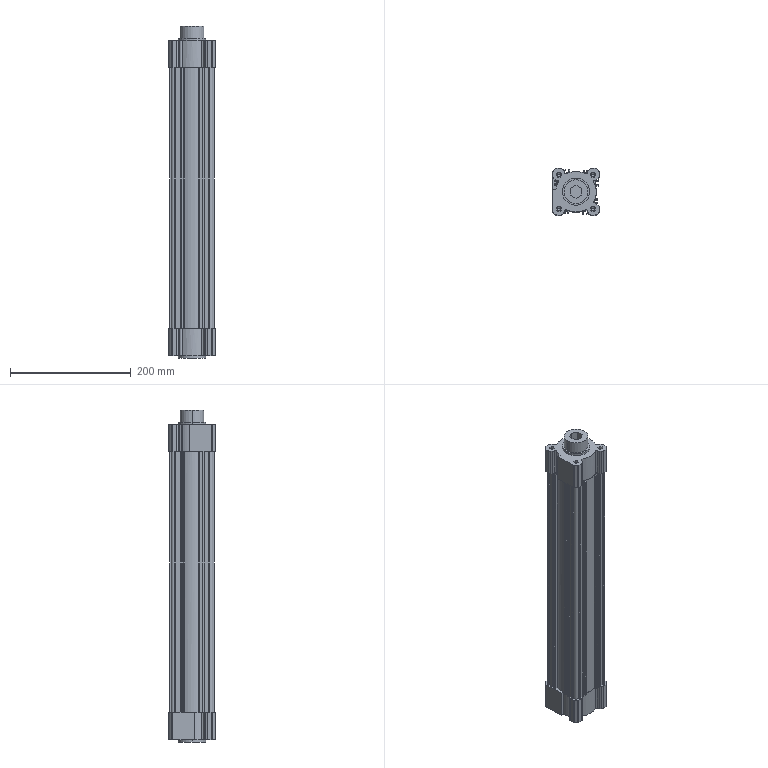Part | SolidWorks | features BaseBody 1 | 1 solid | 409 faces | box 77 x 77 x 549 mm | volume 1158524 mm3 | plane 257 | cylinder 120 | cone 32 | commonest cylinder face diameters 8 x30 4 x17 6.647 x16 20 x14 4.25 x9 67 x9